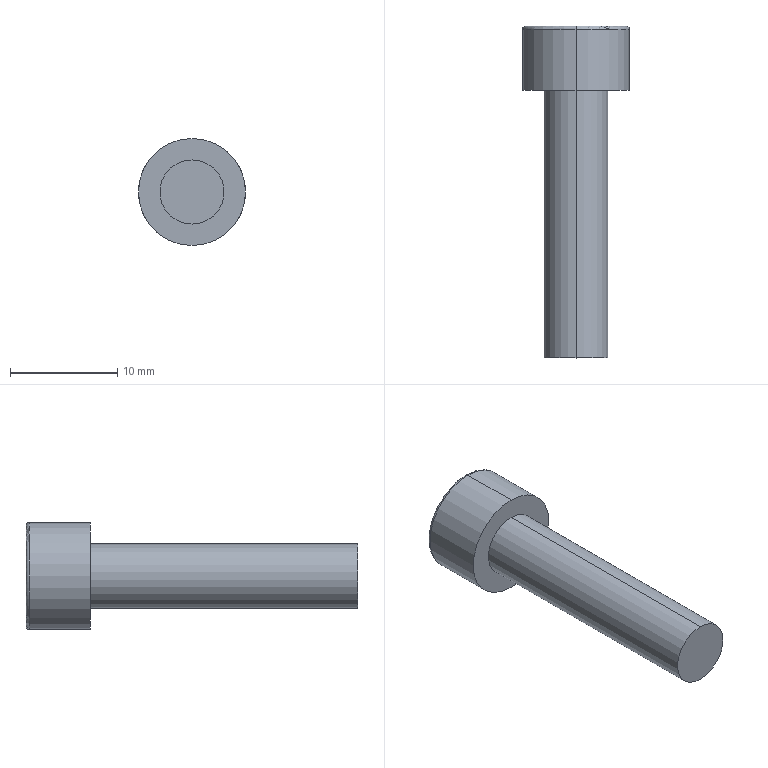Part | STEP file | M6 socket head cap screw simplified_M6x25 | 1 solid | 16 faces | box 10 x 31 x 10 mm | volume 1110 mm3 | plane 10 | cylinder 4 | torus 2 | commonest cylinder face diameters 6 x2 10 x2
STEP:
#1=CARTESIAN_POINT('',(0.,0.,0.));
#2=DIRECTION('',(0.,0.,1.));
#3=DIRECTION('',(1.,0.,0.));
#4=AXIS2_PLACEMENT_3D('',#1,#2,#3);
#5=CARTESIAN_POINT('',(0.,0.,4.7));
#6=VERTEX_POINT('',#5);
#7=CARTESIAN_POINT('',(0.,0.,-4.7));
#8=VERTEX_POINT('',#7);
#9=CARTESIAN_POINT('',(0.,0.,0.));
#10=DIRECTION('',(0.,1.,0.));
#11=DIRECTION('',(0.,0.,-1.));
#12=AXIS2_PLACEMENT_3D('',#9,#10,#11);
#13=CIRCLE('',#12,4.7);
#14=CARTESIAN_POINT('',(0.,-0.3,0.));
#15=DIRECTION('',(0.,-1.,0.));
#16=DIRECTION('',(0.,0.,-1.));
#17=AXIS2_PLACEMENT_3D('',#14,#15,#16);
#18=TOROIDAL_SURFACE('',#17,4.7,0.3);
#19=CARTESIAN_POINT('',(6.283,4.712));
#20=DIRECTION('',(-1.,0.));
#21=VECTOR('',#20,1.);
#22=LINE('',#19,#21);
#23=(GEOMETRIC_REPRESENTATION_CONTEXT(2)PARAMETRIC_REPRESENTATION_CONTEXT()REPRESENTATION_CONTEXT('',''));
#24=DEFINITIONAL_REPRESENTATION('',(#22),#23);
#25=PCURVE('',#18,#24);
#26=CARTESIAN_POINT('',(0.,0.,0.));
#27=DIRECTION('',(0.,-1.,0.));
#28=DIRECTION('',(0.,0.,-1.));
#29=AXIS2_PLACEMENT_3D('',#26,#27,#28);
#30=PLANE('',#29);
#31=CARTESIAN_POINT('',(4.7,0.));
#32=CARTESIAN_POINT('',(4.7,-8.141));
#33=CARTESIAN_POINT('',(-2.35,-4.07));
#34=CARTESIAN_POINT('',(-9.4,0.));
#35=CARTESIAN_POINT('',(-2.35,4.07));
#36=CARTESIAN_POINT('',(4.7,8.141));
#37=CARTESIAN_POINT('',(4.7,0.));
#38=(BOUNDED_CURVE()B_SPLINE_CURVE(2,(#31,#32,#33,#34,#35,#36,#37),.UNSPECIFIED.,.T.,.F.)B_SPLINE_CURVE_WITH_KNOTS((1,2,2,2,2,1),(-2.094,0.,2.094,4.189,6.283,8.378),.UNSPECIFIED.)CURVE()GEOMETRIC_REPRESENTATION_ITEM()RATIONAL_B_SPLINE_CURVE((1.,0.5,1.,0.5,1.,0.5,1.))REPRESENTATION_ITEM(''));
#39=(GEOMETRIC_REPRESENTATION_CONTEXT(2)PARAMETRIC_REPRESENTATION_CONTEXT()REPRESENTATION_CONTEXT('',''));
#40=DEFINITIONAL_REPRESENTATION('',(#38),#39);
#41=PCURVE('',#30,#40);
#42=SURFACE_CURVE('',#13,(#25,#41),.PCURVE_S1.);
#43=EDGE_CURVE('',#6,#8,#42,.T.);
#44=ORIENTED_EDGE('',*,*,#43,.F.);
#45=CARTESIAN_POINT('',(0.,-0.3,5.));
#46=VERTEX_POINT('',#45);
#47=CARTESIAN_POINT('',(0.,-0.3,4.7));
#48=DIRECTION('',(1.,0.,0.));
#49=DIRECTION('',(0.,0.,-1.));
#50=AXIS2_PLACEMENT_3D('',#47,#48,#49);
#51=CIRCLE('',#50,0.3);
#52=CARTESIAN_POINT('',(3.142,3.142));
#53=DIRECTION('',(0.,1.));
#54=VECTOR('',#53,1.);
#55=LINE('',#52,#54);
#56=(GEOMETRIC_REPRESENTATION_CONTEXT(2)PARAMETRIC_REPRESENTATION_CONTEXT()REPRESENTATION_CONTEXT('',''));
#57=DEFINITIONAL_REPRESENTATION('',(#55),#56);
#58=PCURVE('',#18,#57);
#59=CARTESIAN_POINT('',(0.,-0.3,0.));
#60=DIRECTION('',(0.,-1.,0.));
#61=DIRECTION('',(0.,0.,-1.));
#62=AXIS2_PLACEMENT_3D('',#59,#60,#61);
#63=TOROIDAL_SURFACE('',#62,4.7,0.3);
#64=CARTESIAN_POINT('',(3.142,3.142));
#65=DIRECTION('',(0.,1.));
#66=VECTOR('',#65,1.);
#67=LINE('',#64,#66);
#68=(GEOMETRIC_REPRESENTATION_CONTEXT(2)PARAMETRIC_REPRESENTATION_CONTEXT()REPRESENTATION_CONTEXT('',''));
#69=DEFINITIONAL_REPRESENTATION('',(#67),#68);
#70=PCURVE('',#63,#69);
#71=SURFACE_CURVE('',#51,(#58,#70),.PCURVE_S1.);
#72=EDGE_CURVE('',#6,#46,#71,.T.);
#73=ORIENTED_EDGE('',*,*,#72,.T.);
#74=CARTESIAN_POINT('',(0.,-0.3,-5.));
#75=VERTEX_POINT('',#74);
#76=CARTESIAN_POINT('',(0.,-0.3,0.));
#77=DIRECTION('',(0.,-1.,0.));
#78=DIRECTION('',(0.,0.,-1.));
#79=AXIS2_PLACEMENT_3D('',#76,#77,#78);
#80=CIRCLE('',#79,5.);
#81=CARTESIAN_POINT('',(0.,6.283));
#82=DIRECTION('',(1.,0.));
#83=VECTOR('',#82,1.);
#84=LINE('',#81,#83);
#85=(GEOMETRIC_REPRESENTATION_CONTEXT(2)PARAMETRIC_REPRESENTATION_CONTEXT()REPRESENTATION_CONTEXT('',''));
#86=DEFINITIONAL_REPRESENTATION('',(#84),#85);
#87=PCURVE('',#18,#86);
#88=CARTESIAN_POINT('',(0.,0.,0.));
#89=DIRECTION('',(0.,1.,0.));
#90=DIRECTION('',(0.,0.,1.));
#91=AXIS2_PLACEMENT_3D('',#88,#89,#90);
#92=CYLINDRICAL_SURFACE('',#91,5.);
#93=CARTESIAN_POINT('',(3.142,-0.3));
#94=DIRECTION('',(-1.,0.));
#95=VECTOR('',#94,1.);
#96=LINE('',#93,#95);
#97=(GEOMETRIC_REPRESENTATION_CONTEXT(2)PARAMETRIC_REPRESENTATION_CONTEXT()REPRESENTATION_CONTEXT('',''));
#98=DEFINITIONAL_REPRESENTATION('',(#96),#97);
#99=PCURVE('',#92,#98);
#100=SURFACE_CURVE('',#80,(#87,#99),.PCURVE_S1.);
#101=EDGE_CURVE('',#75,#46,#100,.T.);
#102=ORIENTED_EDGE('',*,*,#101,.F.);
#103=CARTESIAN_POINT('',(0.,-0.3,-4.7));
#104=DIRECTION('',(-1.,0.,0.));
#105=DIRECTION('',(0.,0.,1.));
#106=AXIS2_PLACEMENT_3D('',#103,#104,#105);
#107=CIRCLE('',#106,0.3);
#108=CARTESIAN_POINT('',(0.,3.142));
#109=DIRECTION('',(0.,1.));
#110=VECTOR('',#109,1.);
#111=LINE('',#108,#110);
#112=(GEOMETRIC_REPRESENTATION_CONTEXT(2)PARAMETRIC_REPRESENTATION_CONTEXT()REPRESENTATION_CONTEXT('',''));
#113=DEFINITIONAL_REPRESENTATION('',(#111),#112);
#114=PCURVE('',#18,#113);
#115=CARTESIAN_POINT('',(6.283,3.142));
#116=DIRECTION('',(0.,1.));
#117=VECTOR('',#116,1.);
#118=LINE('',#115,#117);
#119=(GEOMETRIC_REPRESENTATION_CONTEXT(2)PARAMETRIC_REPRESENTATION_CONTEXT()REPRESENTATION_CONTEXT('',''));
#120=DEFINITIONAL_REPRESENTATION('',(#118),#119);
#121=PCURVE('',#63,#120);
#122=SURFACE_CURVE('',#107,(#114,#121),.PCURVE_S1.);
#123=EDGE_CURVE('',#8,#75,#122,.T.);
#124=ORIENTED_EDGE('',*,*,#123,.F.);
#125=EDGE_LOOP('',(#44,#73,#102,#124));
#126=FACE_BOUND('',#125,.T.);
#127=ADVANCED_FACE('',(#126),#18,.T.);
#128=CARTESIAN_POINT('',(0.,-31.,3.));
#129=VERTEX_POINT('',#128);
#130=CARTESIAN_POINT('',(0.,-31.,-3.));
#131=VERTEX_POINT('',#130);
#132=CARTESIAN_POINT('',(0.,-31.,0.));
#133=DIRECTION('',(0.,1.,0.));
#134=DIRECTION('',(0.,0.,1.));
#135=AXIS2_PLACEMENT_3D('',#132,#133,#134);
#136=CIRCLE('',#135,3.);
#137=CARTESIAN_POINT('',(0.,0.,0.));
#138=DIRECTION('',(0.,1.,0.));
#139=DIRECTION('',(0.,0.,1.));
#140=AXIS2_PLACEMENT_3D('',#137,#138,#139);
#141=CYLINDRICAL_SURFACE('',#140,3.);
#142=CARTESIAN_POINT('',(0.,-31.));
#143=DIRECTION('',(1.,0.));
#144=VECTOR('',#143,1.);
#145=LINE('',#142,#144);
#146=(GEOMETRIC_REPRESENTATION_CONTEXT(2)PARAMETRIC_REPRESENTATION_CONTEXT()REPRESENTATION_CONTEXT('',''));
#147=DEFINITIONAL_REPRESENTATION('',(#145),#146);
#148=PCURVE('',#141,#147);
#149=CARTESIAN_POINT('',(3.,-31.,0.));
#150=DIRECTION('',(0.,1.,0.));
#151=DIRECTION('',(0.,0.,1.));
#152=AXIS2_PLACEMENT_3D('',#149,#150,#151);
#153=PLANE('',#152);
#154=CARTESIAN_POINT('',(0.,-3.));
#155=DIRECTION('',(1.,0.));
#156=AXIS2_PLACEMENT_2D('',#154,#155);
#157=CIRCLE('',#156,3.);
#158=(GEOMETRIC_REPRESENTATION_CONTEXT(2)PARAMETRIC_REPRESENTATION_CONTEXT()REPRESENTATION_CONTEXT('',''));
#159=DEFINITIONAL_REPRESENTATION('',(#157),#158);
#160=PCURVE('',#153,#159);
#161=SURFACE_CURVE('',#136,(#148,#160),.PCURVE_S1.);
#162=EDGE_CURVE('',#129,#131,#161,.T.);
#163=ORIENTED_EDGE('',*,*,#162,.T.);
#164=CARTESIAN_POINT('',(0.,-6.,-3.));
#165=VERTEX_POINT('',#164);
#166=CARTESIAN_POINT('',(0.,0.,-3.));
#167=DIRECTION('',(0.,1.,0.));
#168=VECTOR('',#167,1.);
#169=LINE('',#166,#168);
#170=CARTESIAN_POINT('',(3.142,0.));
#171=DIRECTION('',(0.,1.));
#172=VECTOR('',#171,1.);
#173=LINE('',#170,#172);
#174=(GEOMETRIC_REPRESENTATION_CONTEXT(2)PARAMETRIC_REPRESENTATION_CONTEXT()REPRESENTATION_CONTEXT('',''));
#175=DEFINITIONAL_REPRESENTATION('',(#173),#174);
#176=PCURVE('',#141,#175);
#177=CARTESIAN_POINT('',(0.,0.,0.));
#178=DIRECTION('',(0.,1.,0.));
#179=DIRECTION('',(0.,0.,1.));
#180=AXIS2_PLACEMENT_3D('',#177,#178,#179);
#181=CYLINDRICAL_SURFACE('',#180,3.);
#182=CARTESIAN_POINT('',(3.142,0.));
#183=DIRECTION('',(0.,1.));
#184=VECTOR('',#183,1.);
#185=LINE('',#182,#184);
#186=(GEOMETRIC_REPRESENTATION_CONTEXT(2)PARAMETRIC_REPRESENTATION_CONTEXT()REPRESENTATION_CONTEXT('',''));
#187=DEFINITIONAL_REPRESENTATION('',(#185),#186);
#188=PCURVE('',#181,#187);
#189=SURFACE_CURVE('',#169,(#176,#188),.PCURVE_S1.);
#190=EDGE_CURVE('',#131,#165,#189,.T.);
#191=ORIENTED_EDGE('',*,*,#190,.T.);
#192=CARTESIAN_POINT('',(0.,-6.,3.));
#193=VERTEX_POINT('',#192);
#194=CARTESIAN_POINT('',(0.,-6.,0.));
#195=DIRECTION('',(0.,1.,0.));
#196=DIRECTION('',(0.,0.,1.));
#197=AXIS2_PLACEMENT_3D('',#194,#195,#196);
#198=CIRCLE('',#197,3.);
#199=CARTESIAN_POINT('',(0.,-6.));
#200=DIRECTION('',(1.,0.));
#201=VECTOR('',#200,1.);
#202=LINE('',#199,#201);
#203=(GEOMETRIC_REPRESENTATION_CONTEXT(2)PARAMETRIC_REPRESENTATION_CONTEXT()REPRESENTATION_CONTEXT('',''));
#204=DEFINITIONAL_REPRESENTATION('',(#202),#203);
#205=PCURVE('',#141,#204);
#206=CARTESIAN_POINT('',(5.,-6.,0.));
#207=DIRECTION('',(0.,1.,0.));
#208=DIRECTION('',(0.,0.,1.));
#209=AXIS2_PLACEMENT_3D('',#206,#207,#208);
#210=PLANE('',#209);
#211=CARTESIAN_POINT('',(0.,-5.));
#212=DIRECTION('',(1.,0.));
#213=AXIS2_PLACEMENT_2D('',#211,#212);
#214=CIRCLE('',#213,3.);
#215=(GEOMETRIC_REPRESENTATION_CONTEXT(2)PARAMETRIC_REPRESENTATION_CONTEXT()REPRESENTATION_CONTEXT('',''));
#216=DEFINITIONAL_REPRESENTATION('',(#214),#215);
#217=PCURVE('',#210,#216);
#218=SURFACE_CURVE('',#198,(#205,#217),.PCURVE_S1.);
#219=EDGE_CURVE('',#193,#165,#218,.T.);
#220=ORIENTED_EDGE('',*,*,#219,.F.);
#221=CARTESIAN_POINT('',(0.,0.,3.));
#222=DIRECTION('',(0.,1.,0.));
#223=VECTOR('',#222,1.);
#224=LINE('',#221,#223);
#225=CARTESIAN_POINT('',(0.,0.));
#226=DIRECTION('',(0.,1.));
#227=VECTOR('',#226,1.);
#228=LINE('',#225,#227);
#229=(GEOMETRIC_REPRESENTATION_CONTEXT(2)PARAMETRIC_REPRESENTATION_CONTEXT()REPRESENTATION_CONTEXT('',''));
#230=DEFINITIONAL_REPRESENTATION('',(#228),#229);
#231=PCURVE('',#141,#230);
#232=CARTESIAN_POINT('',(6.283,0.));
#233=DIRECTION('',(0.,1.));
#234=VECTOR('',#233,1.);
#235=LINE('',#232,#234);
#236=(GEOMETRIC_REPRESENTATION_CONTEXT(2)PARAMETRIC_REPRESENTATION_CONTEXT()REPRESENTATION_CONTEXT('',''));
#237=DEFINITIONAL_REPRESENTATION('',(#235),#236);
#238=PCURVE('',#181,#237);
#239=SURFACE_CURVE('',#224,(#231,#238),.PCURVE_S1.);
#240=EDGE_CURVE('',#129,#193,#239,.T.);
#241=ORIENTED_EDGE('',*,*,#240,.F.);
#242=EDGE_LOOP('',(#163,#191,#220,#241));
#243=FACE_BOUND('',#242,.T.);
#244=ADVANCED_FACE('',(#243),#141,.T.);
#245=CARTESIAN_POINT('',(0.,-6.,5.));
#246=VERTEX_POINT('',#245);
#247=CARTESIAN_POINT('',(0.,-6.,-5.));
#248=VERTEX_POINT('',#247);
#249=CARTESIAN_POINT('',(0.,-6.,0.));
#250=DIRECTION('',(0.,1.,0.));
#251=DIRECTION('',(0.,0.,1.));
#252=AXIS2_PLACEMENT_3D('',#249,#250,#251);
#253=CIRCLE('',#252,5.);
#254=CARTESIAN_POINT('',(0.,-6.));
#255=DIRECTION('',(1.,0.));
#256=VECTOR('',#255,1.);
#257=LINE('',#254,#256);
#258=(GEOMETRIC_REPRESENTATION_CONTEXT(2)PARAMETRIC_REPRESENTATION_CONTEXT()REPRESENTATION_CONTEXT('',''));
#259=DEFINITIONAL_REPRESENTATION('',(#257),#258);
#260=PCURVE('',#92,#259);
#261=CARTESIAN_POINT('',(0.,-5.));
#262=DIRECTION('',(1.,0.));
#263=AXIS2_PLACEMENT_2D('',#261,#262);
#264=CIRCLE('',#263,5.);
#265=(GEOMETRIC_REPRESENTATION_CONTEXT(2)PARAMETRIC_REPRESENTATION_CONTEXT()REPRESENTATION_CONTEXT('',''));
#266=DEFINITIONAL_REPRESENTATION('',(#264),#265);
#267=PCURVE('',#210,#266);
#268=SURFACE_CURVE('',#253,(#260,#267),.PCURVE_S1.);
#269=EDGE_CURVE('',#246,#248,#268,.T.);
#270=ORIENTED_EDGE('',*,*,#269,.T.);
#271=CARTESIAN_POINT('',(0.,0.,-5.));
#272=DIRECTION('',(0.,1.,0.));
#273=VECTOR('',#272,1.);
#274=LINE('',#271,#273);
#275=CARTESIAN_POINT('',(3.142,0.));
#276=DIRECTION('',(0.,1.));
#277=VECTOR('',#276,1.);
#278=LINE('',#275,#277);
#279=(GEOMETRIC_REPRESENTATION_CONTEXT(2)PARAMETRIC_REPRESENTATION_CONTEXT()REPRESENTATION_CONTEXT('',''));
#280=DEFINITIONAL_REPRESENTATION('',(#278),#279);
#281=PCURVE('',#92,#280);
#282=CARTESIAN_POINT('',(0.,0.,0.));
#283=DIRECTION('',(0.,1.,0.));
#284=DIRECTION('',(0.,0.,1.));
#285=AXIS2_PLACEMENT_3D('',#282,#283,#284);
#286=CYLINDRICAL_SURFACE('',#285,5.);
#287=CARTESIAN_POINT('',(3.142,0.));
#288=DIRECTION('',(0.,1.));
#289=VECTOR('',#288,1.);
#290=LINE('',#287,#289);
#291=(GEOMETRIC_REPRESENTATION_CONTEXT(2)PARAMETRIC_REPRESENTATION_CONTEXT()REPRESENTATION_CONTEXT('',''));
#292=DEFINITIONAL_REPRESENTATION('',(#290),#291);
#293=PCURVE('',#286,#292);
#294=SURFACE_CURVE('',#274,(#281,#293),.PCURVE_S1.);
#295=EDGE_CURVE('',#248,#75,#294,.T.);
#296=ORIENTED_EDGE('',*,*,#295,.T.);
#297=ORIENTED_EDGE('',*,*,#101,.T.);
#298=CARTESIAN_POINT('',(0.,0.,5.));
#299=DIRECTION('',(0.,1.,0.));
#300=VECTOR('',#299,1.);
#301=LINE('',#298,#300);
#302=CARTESIAN_POINT('',(0.,0.));
#303=DIRECTION('',(0.,1.));
#304=VECTOR('',#303,1.);
#305=LINE('',#302,#304);
#306=(GEOMETRIC_REPRESENTATION_CONTEXT(2)PARAMETRIC_REPRESENTATION_CONTEXT()REPRESENTATION_CONTEXT('',''));
#307=DEFINITIONAL_REPRESENTATION('',(#305),#306);
#308=PCURVE('',#92,#307);
#309=CARTESIAN_POINT('',(6.283,0.));
#310=DIRECTION('',(0.,1.));
#311=VECTOR('',#310,1.);
#312=LINE('',#309,#311);
#313=(GEOMETRIC_REPRESENTATION_CONTEXT(2)PARAMETRIC_REPRESENTATION_CONTEXT()REPRESENTATION_CONTEXT('',''));
#314=DEFINITIONAL_REPRESENTATION('',(#312),#313);
#315=PCURVE('',#286,#314);
#316=SURFACE_CURVE('',#301,(#308,#315),.PCURVE_S1.);
#317=EDGE_CURVE('',#246,#46,#316,.T.);
#318=ORIENTED_EDGE('',*,*,#317,.F.);
#319=EDGE_LOOP('',(#270,#296,#297,#318));
#320=FACE_BOUND('',#319,.T.);
#321=ADVANCED_FACE('',(#320),#92,.T.);
#322=CARTESIAN_POINT('',(0.,0.,0.));
#323=DIRECTION('',(0.,1.,0.));
#324=DIRECTION('',(0.,0.,-1.));
#325=AXIS2_PLACEMENT_3D('',#322,#323,#324);
#326=CIRCLE('',#325,4.7);
#327=CARTESIAN_POINT('',(4.7,0.));
#328=CARTESIAN_POINT('',(4.7,-8.141));
#329=CARTESIAN_POINT('',(-2.35,-4.07));
#330=CARTESIAN_POINT('',(-9.4,0.));
#331=CARTESIAN_POINT('',(-2.35,4.07));
#332=CARTESIAN_POINT('',(4.7,8.141));
#333=CARTESIAN_POINT('',(4.7,0.));
#334=(BOUNDED_CURVE()B_SPLINE_CURVE(2,(#327,#328,#329,#330,#331,#332,#333),.UNSPECIFIED.,.T.,.F.)B_SPLINE_CURVE_WITH_KNOTS((1,2,2,2,2,1),(-2.094,0.,2.094,4.189,6.283,8.378),.UNSPECIFIED.)CURVE()GEOMETRIC_REPRESENTATION_ITEM()RATIONAL_B_SPLINE_CURVE((1.,0.5,1.,0.5,1.,0.5,1.))REPRESENTATION_ITEM(''));
#335=(GEOMETRIC_REPRESENTATION_CONTEXT(2)PARAMETRIC_REPRESENTATION_CONTEXT()REPRESENTATION_CONTEXT('',''));
#336=DEFINITIONAL_REPRESENTATION('',(#334),#335);
#337=PCURVE('',#30,#336);
#338=CARTESIAN_POINT('',(6.283,4.712));
#339=DIRECTION('',(-1.,0.));
#340=VECTOR('',#339,1.);
#341=LINE('',#338,#340);
#342=(GEOMETRIC_REPRESENTATION_CONTEXT(2)PARAMETRIC_REPRESENTATION_CONTEXT()REPRESENTATION_CONTEXT('',''));
#343=DEFINITIONAL_REPRESENTATION('',(#341),#342);
#344=PCURVE('',#63,#343);
#345=SURFACE_CURVE('',#326,(#337,#344),.PCURVE_S1.);
#346=EDGE_CURVE('',#8,#6,#345,.T.);
#347=ORIENTED_EDGE('',*,*,#346,.T.);
#348=ORIENTED_EDGE('',*,*,#43,.T.);
#349=EDGE_LOOP('',(#347,#348));
#350=FACE_BOUND('',#349,.T.);
#351=CARTESIAN_POINT('',(-2.944,0.,0.));
#352=VERTEX_POINT('',#351);
#353=CARTESIAN_POINT('',(-1.472,0.,2.55));
#354=VERTEX_POINT('',#353);
#355=CARTESIAN_POINT('',(-2.944,0.,0.));
#356=DIRECTION('',(0.5,0.,0.866));
#357=VECTOR('',#356,1.);
#358=LINE('',#355,#357);
#359=CARTESIAN_POINT('',(0.,-2.944));
#360=DIRECTION('',(-0.866,0.5));
#361=VECTOR('',#360,1.);
#362=LINE('',#359,#361);
#363=(GEOMETRIC_REPRESENTATION_CONTEXT(2)PARAMETRIC_REPRESENTATION_CONTEXT()REPRESENTATION_CONTEXT('',''));
#364=DEFINITIONAL_REPRESENTATION('',(#362),#363);
#365=PCURVE('',#30,#364);
#366=CARTESIAN_POINT('',(-2.944,-3.,0.));
#367=DIRECTION('',(-0.866,0.,0.5));
#368=DIRECTION('',(0.5,0.,0.866));
#369=AXIS2_PLACEMENT_3D('',#366,#367,#368);
#370=PLANE('',#369);
#371=CARTESIAN_POINT('',(0.,3.));
#372=DIRECTION('',(1.,0.));
#373=VECTOR('',#372,1.);
#374=LINE('',#371,#373);
#375=(GEOMETRIC_REPRESENTATION_CONTEXT(2)PARAMETRIC_REPRESENTATION_CONTEXT()REPRESENTATION_CONTEXT('',''));
#376=DEFINITIONAL_REPRESENTATION('',(#374),#375);
#377=PCURVE('',#370,#376);
#378=SURFACE_CURVE('',#358,(#365,#377),.PCURVE_S1.);
#379=EDGE_CURVE('',#352,#354,#378,.T.);
#380=ORIENTED_EDGE('',*,*,#379,.F.);
#381=CARTESIAN_POINT('',(-1.472,0.,-2.55));
#382=VERTEX_POINT('',#381);
#383=CARTESIAN_POINT('',(-1.472,0.,-2.55));
#384=DIRECTION('',(-0.5,0.,0.866));
#385=VECTOR('',#384,1.);
#386=LINE('',#383,#385);
#387=CARTESIAN_POINT('',(2.55,-1.472));
#388=DIRECTION('',(-0.866,-0.5));
#389=VECTOR('',#388,1.);
#390=LINE('',#387,#389);
#391=(GEOMETRIC_REPRESENTATION_CONTEXT(2)PARAMETRIC_REPRESENTATION_CONTEXT()REPRESENTATION_CONTEXT('',''));
#392=DEFINITIONAL_REPRESENTATION('',(#390),#391);
#393=PCURVE('',#30,#392);
#394=CARTESIAN_POINT('',(-1.472,-3.,-2.55));
#395=DIRECTION('',(-0.866,0.,-0.5));
#396=DIRECTION('',(-0.5,0.,0.866));
#397=AXIS2_PLACEMENT_3D('',#394,#395,#396);
#398=PLANE('',#397);
#399=CARTESIAN_POINT('',(0.,3.));
#400=DIRECTION('',(1.,0.));
#401=VECTOR('',#400,1.);
#402=LINE('',#399,#401);
#403=(GEOMETRIC_REPRESENTATION_CONTEXT(2)PARAMETRIC_REPRESENTATION_CONTEXT()REPRESENTATION_CONTEXT('',''));
#404=DEFINITIONAL_REPRESENTATION('',(#402),#403);
#405=PCURVE('',#398,#404);
#406=SURFACE_CURVE('',#386,(#393,#405),.PCURVE_S1.);
#407=EDGE_CURVE('',#382,#352,#406,.T.);
#408=ORIENTED_EDGE('',*,*,#407,.F.);
#409=CARTESIAN_POINT('',(1.472,0.,-2.55));
#410=VERTEX_POINT('',#409);
#411=CARTESIAN_POINT('',(1.472,0.,-2.55));
#412=DIRECTION('',(-1.,0.,0.));
#413=VECTOR('',#412,1.);
#414=LINE('',#411,#413);
#415=CARTESIAN_POINT('',(2.55,1.472));
#416=DIRECTION('',(0.,-1.));
#417=VECTOR('',#416,1.);
#418=LINE('',#415,#417);
#419=(GEOMETRIC_REPRESENTATION_CONTEXT(2)PARAMETRIC_REPRESENTATION_CONTEXT()REPRESENTATION_CONTEXT('',''));
#420=DEFINITIONAL_REPRESENTATION('',(#418),#419);
#421=PCURVE('',#30,#420);
#422=CARTESIAN_POINT('',(1.472,-3.,-2.55));
#423=DIRECTION('',(0.,0.,-1.));
#424=DIRECTION('',(-1.,0.,0.));
#425=AXIS2_PLACEMENT_3D('',#422,#423,#424);
#426=PLANE('',#425);
#427=CARTESIAN_POINT('',(0.,3.));
#428=DIRECTION('',(1.,0.));
#429=VECTOR('',#428,1.);
#430=LINE('',#427,#429);
#431=(GEOMETRIC_REPRESENTATION_CONTEXT(2)PARAMETRIC_REPRESENTATION_CONTEXT()REPRESENTATION_CONTEXT('',''));
#432=DEFINITIONAL_REPRESENTATION('',(#430),#431);
#433=PCURVE('',#426,#432);
#434=SURFACE_CURVE('',#414,(#421,#433),.PCURVE_S1.);
#435=EDGE_CURVE('',#410,#382,#434,.T.);
#436=ORIENTED_EDGE('',*,*,#435,.F.);
#437=CARTESIAN_POINT('',(2.944,0.,0.));
#438=VERTEX_POINT('',#437);
#439=CARTESIAN_POINT('',(2.944,0.,0.));
#440=DIRECTION('',(-0.5,0.,-0.866));
#441=VECTOR('',#440,1.);
#442=LINE('',#439,#441);
#443=CARTESIAN_POINT('',(0.,2.944));
#444=DIRECTION('',(0.866,-0.5));
#445=VECTOR('',#444,1.);
#446=LINE('',#443,#445);
#447=(GEOMETRIC_REPRESENTATION_CONTEXT(2)PARAMETRIC_REPRESENTATION_CONTEXT()REPRESENTATION_CONTEXT('',''));
#448=DEFINITIONAL_REPRESENTATION('',(#446),#447);
#449=PCURVE('',#30,#448);
#450=CARTESIAN_POINT('',(2.944,-3.,0.));
#451=DIRECTION('',(0.866,0.,-0.5));
#452=DIRECTION('',(-0.5,0.,-0.866));
#453=AXIS2_PLACEMENT_3D('',#450,#451,#452);
#454=PLANE('',#453);
#455=CARTESIAN_POINT('',(0.,3.));
#456=DIRECTION('',(1.,0.));
#457=VECTOR('',#456,1.);
#458=LINE('',#455,#457);
#459=(GEOMETRIC_REPRESENTATION_CONTEXT(2)PARAMETRIC_REPRESENTATION_CONTEXT()REPRESENTATION_CONTEXT('',''));
#460=DEFINITIONAL_REPRESENTATION('',(#458),#459);
#461=PCURVE('',#454,#460);
#462=SURFACE_CURVE('',#442,(#449,#461),.PCURVE_S1.);
#463=EDGE_CURVE('',#438,#410,#462,.T.);
#464=ORIENTED_EDGE('',*,*,#463,.F.);
#465=CARTESIAN_POINT('',(1.472,0.,2.55));
#466=VERTEX_POINT('',#465);
#467=CARTESIAN_POINT('',(1.472,0.,2.55));
#468=DIRECTION('',(0.5,0.,-0.866));
#469=VECTOR('',#468,1.);
#470=LINE('',#467,#469);
#471=CARTESIAN_POINT('',(-2.55,1.472));
#472=DIRECTION('',(0.866,0.5));
#473=VECTOR('',#472,1.);
#474=LINE('',#471,#473);
#475=(GEOMETRIC_REPRESENTATION_CONTEXT(2)PARAMETRIC_REPRESENTATION_CONTEXT()REPRESENTATION_CONTEXT('',''));
#476=DEFINITIONAL_REPRESENTATION('',(#474),#475);
#477=PCURVE('',#30,#476);
#478=CARTESIAN_POINT('',(1.472,-3.,2.55));
#479=DIRECTION('',(0.866,0.,0.5));
#480=DIRECTION('',(0.5,0.,-0.866));
#481=AXIS2_PLACEMENT_3D('',#478,#479,#480);
#482=PLANE('',#481);
#483=CARTESIAN_POINT('',(0.,3.));
#484=DIRECTION('',(1.,0.));
#485=VECTOR('',#484,1.);
#486=LINE('',#483,#485);
#487=(GEOMETRIC_REPRESENTATION_CONTEXT(2)PARAMETRIC_REPRESENTATION_CONTEXT()REPRESENTATION_CONTEXT('',''));
#488=DEFINITIONAL_REPRESENTATION('',(#486),#487);
#489=PCURVE('',#482,#488);
#490=SURFACE_CURVE('',#470,(#477,#489),.PCURVE_S1.);
#491=EDGE_CURVE('',#466,#438,#490,.T.);
#492=ORIENTED_EDGE('',*,*,#491,.F.);
#493=CARTESIAN_POINT('',(-1.472,0.,2.55));
#494=DIRECTION('',(1.,0.,0.));
#495=VECTOR('',#494,1.);
#496=LINE('',#493,#495);
#497=CARTESIAN_POINT('',(-2.55,-1.472));
#498=DIRECTION('',(0.,1.));
#499=VECTOR('',#498,1.);
#500=LINE('',#497,#499);
#501=(GEOMETRIC_REPRESENTATION_CONTEXT(2)PARAMETRIC_REPRESENTATION_CONTEXT()REPRESENTATION_CONTEXT('',''));
#502=DEFINITIONAL_REPRESENTATION('',(#500),#501);
#503=PCURVE('',#30,#502);
#504=CARTESIAN_POINT('',(-1.472,-3.,2.55));
#505=DIRECTION('',(0.,0.,1.));
#506=DIRECTION('',(1.,0.,0.));
#507=AXIS2_PLACEMENT_3D('',#504,#505,#506);
#508=PLANE('',#507);
#509=CARTESIAN_POINT('',(0.,3.));
#510=DIRECTION('',(1.,0.));
#511=VECTOR('',#510,1.);
#512=LINE('',#509,#511);
#513=(GEOMETRIC_REPRESENTATION_CONTEXT(2)PARAMETRIC_REPRESENTATION_CONTEXT()REPRESENTATION_CONTEXT('',''));
#514=DEFINITIONAL_REPRESENTATION('',(#512),#513);
#515=PCURVE('',#508,#514);
#516=SURFACE_CURVE('',#496,(#503,#515),.PCURVE_S1.);
#517=EDGE_CURVE('',#354,#466,#516,.T.);
#518=ORIENTED_EDGE('',*,*,#517,.F.);
#519=EDGE_LOOP('',(#380,#408,#436,#464,#492,#518));
#520=FACE_BOUND('',#519,.T.);
#521=ADVANCED_FACE('',(#350,#520),#30,.F.);
#522=ORIENTED_EDGE('',*,*,#295,.F.);
#523=CARTESIAN_POINT('',(0.,-6.,0.));
#524=DIRECTION('',(0.,1.,0.));
#525=DIRECTION('',(0.,0.,1.));
#526=AXIS2_PLACEMENT_3D('',#523,#524,#525);
#527=CIRCLE('',#526,5.);
#528=CARTESIAN_POINT('',(0.,-6.));
#529=DIRECTION('',(1.,0.));
#530=VECTOR('',#529,1.);
#531=LINE('',#528,#530);
#532=(GEOMETRIC_REPRESENTATION_CONTEXT(2)PARAMETRIC_REPRESENTATION_CONTEXT()REPRESENTATION_CONTEXT('',''));
#533=DEFINITIONAL_REPRESENTATION('',(#531),#532);
#534=PCURVE('',#286,#533);
#535=CARTESIAN_POINT('',(0.,-5.));
#536=DIRECTION('',(1.,0.));
#537=AXIS2_PLACEMENT_2D('',#535,#536);
#538=CIRCLE('',#537,5.);
#539=(GEOMETRIC_REPRESENTATION_CONTEXT(2)PARAMETRIC_REPRESENTATION_CONTEXT()REPRESENTATION_CONTEXT('',''));
#540=DEFINITIONAL_REPRESENTATION('',(#538),#539);
#541=PCURVE('',#210,#540);
#542=SURFACE_CURVE('',#527,(#534,#541),.PCURVE_S1.);
#543=EDGE_CURVE('',#248,#246,#542,.T.);
#544=ORIENTED_EDGE('',*,*,#543,.T.);
#545=ORIENTED_EDGE('',*,*,#317,.T.);
#546=CARTESIAN_POINT('',(0.,-0.3,0.));
#547=DIRECTION('',(0.,-1.,0.));
#548=DIRECTION('',(0.,0.,-1.));
#549=AXIS2_PLACEMENT_3D('',#546,#547,#548);
#550=CIRCLE('',#549,5.);
#551=CARTESIAN_POINT('',(9.425,-0.3));
#552=DIRECTION('',(-1.,0.));
#553=VECTOR('',#552,1.);
#554=LINE('',#551,#553);
#555=(GEOMETRIC_REPRESENTATION_CONTEXT(2)PARAMETRIC_REPRESENTATION_CONTEXT()REPRESENTATION_CONTEXT('',''));
#556=DEFINITIONAL_REPRESENTATION('',(#554),#555);
#557=PCURVE('',#286,#556);
#558=CARTESIAN_POINT('',(0.,6.283));
#559=DIRECTION('',(1.,0.));
#560=VECTOR('',#559,1.);
#561=LINE('',#558,#560);
#562=(GEOMETRIC_REPRESENTATION_CONTEXT(2)PARAMETRIC_REPRESENTATION_CONTEXT()REPRESENTATION_CONTEXT('',''));
#563=DEFINITIONAL_REPRESENTATION('',(#561),#562);
#564=PCURVE('',#63,#563);
#565=SURFACE_CURVE('',#550,(#557,#564),.PCURVE_S1.);
#566=EDGE_CURVE('',#46,#75,#565,.T.);
#567=ORIENTED_EDGE('',*,*,#566,.T.);
#568=EDGE_LOOP('',(#522,#544,#545,#567));
#569=FACE_BOUND('',#568,.T.);
#570=ADVANCED_FACE('',(#569),#286,.T.);
#571=ORIENTED_EDGE('',*,*,#269,.F.);
#572=ORIENTED_EDGE('',*,*,#543,.F.);
#573=EDGE_LOOP('',(#571,#572));
#574=FACE_BOUND('',#573,.T.);
#575=ORIENTED_EDGE('',*,*,#219,.T.);
#576=CARTESIAN_POINT('',(0.,-6.,0.));
#577=DIRECTION('',(0.,1.,0.));
#578=DIRECTION('',(0.,0.,1.));
#579=AXIS2_PLACEMENT_3D('',#576,#577,#578);
#580=CIRCLE('',#579,3.);
#581=CARTESIAN_POINT('',(0.,-5.));
#582=DIRECTION('',(1.,0.));
#583=AXIS2_PLACEMENT_2D('',#581,#582);
#584=CIRCLE('',#583,3.);
#585=(GEOMETRIC_REPRESENTATION_CONTEXT(2)PARAMETRIC_REPRESENTATION_CONTEXT()REPRESENTATION_CONTEXT('',''));
#586=DEFINITIONAL_REPRESENTATION('',(#584),#585);
#587=PCURVE('',#210,#586);
#588=CARTESIAN_POINT('',(0.,-6.));
#589=DIRECTION('',(1.,0.));
#590=VECTOR('',#589,1.);
#591=LINE('',#588,#590);
#592=(GEOMETRIC_REPRESENTATION_CONTEXT(2)PARAMETRIC_REPRESENTATION_CONTEXT()REPRESENTATION_CONTEXT('',''));
#593=DEFINITIONAL_REPRESENTATION('',(#591),#592);
#594=PCURVE('',#181,#593);
#595=SURFACE_CURVE('',#580,(#587,#594),.PCURVE_S1.);
#596=EDGE_CURVE('',#165,#193,#595,.T.);
#597=ORIENTED_EDGE('',*,*,#596,.T.);
#598=EDGE_LOOP('',(#575,#597));
#599=FACE_BOUND('',#598,.T.);
#600=ADVANCED_FACE('',(#574,#599),#210,.F.);
#601=ORIENTED_EDGE('',*,*,#190,.F.);
#602=CARTESIAN_POINT('',(0.,-31.,0.));
#603=DIRECTION('',(0.,1.,0.));
#604=DIRECTION('',(0.,0.,1.));
#605=AXIS2_PLACEMENT_3D('',#602,#603,#604);
#606=CIRCLE('',#605,3.);
#607=CARTESIAN_POINT('',(0.,-31.));
#608=DIRECTION('',(1.,0.));
#609=VECTOR('',#608,1.);
#610=LINE('',#607,#609);
#611=(GEOMETRIC_REPRESENTATION_CONTEXT(2)PARAMETRIC_REPRESENTATION_CONTEXT()REPRESENTATION_CONTEXT('',''));
#612=DEFINITIONAL_REPRESENTATION('',(#610),#611);
#613=PCURVE('',#181,#612);
#614=CARTESIAN_POINT('',(0.,-3.));
#615=DIRECTION('',(1.,0.));
#616=AXIS2_PLACEMENT_2D('',#614,#615);
#617=CIRCLE('',#616,3.);
#618=(GEOMETRIC_REPRESENTATION_CONTEXT(2)PARAMETRIC_REPRESENTATION_CONTEXT()REPRESENTATION_CONTEXT('',''));
#619=DEFINITIONAL_REPRESENTATION('',(#617),#618);
#620=PCURVE('',#153,#619);
#621=SURFACE_CURVE('',#606,(#613,#620),.PCURVE_S1.);
#622=EDGE_CURVE('',#131,#129,#621,.T.);
#623=ORIENTED_EDGE('',*,*,#622,.T.);
#624=ORIENTED_EDGE('',*,*,#240,.T.);
#625=ORIENTED_EDGE('',*,*,#596,.F.);
#626=EDGE_LOOP('',(#601,#623,#624,#625));
#627=FACE_BOUND('',#626,.T.);
#628=ADVANCED_FACE('',(#627),#181,.T.);
#629=ORIENTED_EDGE('',*,*,#162,.F.);
#630=ORIENTED_EDGE('',*,*,#622,.F.);
#631=EDGE_LOOP('',(#629,#630));
#632=FACE_BOUND('',#631,.T.);
#633=ADVANCED_FACE('',(#632),#153,.F.);
#634=ORIENTED_EDGE('',*,*,#407,.T.);
#635=CARTESIAN_POINT('',(-2.944,-3.,0.));
#636=VERTEX_POINT('',#635);
#637=CARTESIAN_POINT('',(-2.944,-3.,0.));
#638=DIRECTION('',(0.,1.,0.));
#639=VECTOR('',#638,1.);
#640=LINE('',#637,#639);
#641=CARTESIAN_POINT('',(2.944,0.));
#642=DIRECTION('',(0.,1.));
#643=VECTOR('',#642,1.);
#644=LINE('',#641,#643);
#645=(GEOMETRIC_REPRESENTATION_CONTEXT(2)PARAMETRIC_REPRESENTATION_CONTEXT()REPRESENTATION_CONTEXT('',''));
#646=DEFINITIONAL_REPRESENTATION('',(#644),#645);
#647=PCURVE('',#398,#646);
#648=CARTESIAN_POINT('',(0.,0.));
#649=DIRECTION('',(0.,1.));
#650=VECTOR('',#649,1.);
#651=LINE('',#648,#650);
#652=(GEOMETRIC_REPRESENTATION_CONTEXT(2)PARAMETRIC_REPRESENTATION_CONTEXT()REPRESENTATION_CONTEXT('',''));
#653=DEFINITIONAL_REPRESENTATION('',(#651),#652);
#654=PCURVE('',#370,#653);
#655=SURFACE_CURVE('',#640,(#647,#654),.PCURVE_S1.);
#656=EDGE_CURVE('',#636,#352,#655,.T.);
#657=ORIENTED_EDGE('',*,*,#656,.F.);
#658=CARTESIAN_POINT('',(-1.472,-3.,-2.55));
#659=VERTEX_POINT('',#658);
#660=CARTESIAN_POINT('',(-1.472,-3.,-2.55));
#661=DIRECTION('',(-0.5,0.,0.866));
#662=VECTOR('',#661,1.);
#663=LINE('',#660,#662);
#664=CARTESIAN_POINT('',(0.,0.));
#665=DIRECTION('',(1.,0.));
#666=VECTOR('',#665,1.);
#667=LINE('',#664,#666);
#668=(GEOMETRIC_REPRESENTATION_CONTEXT(2)PARAMETRIC_REPRESENTATION_CONTEXT()REPRESENTATION_CONTEXT('',''));
#669=DEFINITIONAL_REPRESENTATION('',(#667),#668);
#670=PCURVE('',#398,#669);
#671=CARTESIAN_POINT('',(-2.944,-3.,0.));
#672=DIRECTION('',(0.,1.,0.));
#673=DIRECTION('',(0.,0.,1.));
#674=AXIS2_PLACEMENT_3D('',#671,#672,#673);
#675=PLANE('',#674);
#676=CARTESIAN_POINT('',(-2.55,1.472));
#677=DIRECTION('',(0.866,-0.5));
#678=VECTOR('',#677,1.);
#679=LINE('',#676,#678);
#680=(GEOMETRIC_REPRESENTATION_CONTEXT(2)PARAMETRIC_REPRESENTATION_CONTEXT()REPRESENTATION_CONTEXT('',''));
#681=DEFINITIONAL_REPRESENTATION('',(#679),#680);
#682=PCURVE('',#675,#681);
#683=SURFACE_CURVE('',#663,(#670,#682),.PCURVE_S1.);
#684=EDGE_CURVE('',#659,#636,#683,.T.);
#685=ORIENTED_EDGE('',*,*,#684,.F.);
#686=CARTESIAN_POINT('',(-1.472,-3.,-2.55));
#687=DIRECTION('',(0.,1.,0.));
#688=VECTOR('',#687,1.);
#689=LINE('',#686,#688);
#690=CARTESIAN_POINT('',(0.,0.));
#691=DIRECTION('',(0.,1.));
#692=VECTOR('',#691,1.);
#693=LINE('',#690,#692);
#694=(GEOMETRIC_REPRESENTATION_CONTEXT(2)PARAMETRIC_REPRESENTATION_CONTEXT()REPRESENTATION_CONTEXT('',''));
#695=DEFINITIONAL_REPRESENTATION('',(#693),#694);
#696=PCURVE('',#398,#695);
#697=CARTESIAN_POINT('',(2.944,0.));
#698=DIRECTION('',(0.,1.));
#699=VECTOR('',#698,1.);
#700=LINE('',#697,#699);
#701=(GEOMETRIC_REPRESENTATION_CONTEXT(2)PARAMETRIC_REPRESENTATION_CONTEXT()REPRESENTATION_CONTEXT('',''));
#702=DEFINITIONAL_REPRESENTATION('',(#700),#701);
#703=PCURVE('',#426,#702);
#704=SURFACE_CURVE('',#689,(#696,#703),.PCURVE_S1.);
#705=EDGE_CURVE('',#659,#382,#704,.T.);
#706=ORIENTED_EDGE('',*,*,#705,.T.);
#707=EDGE_LOOP('',(#634,#657,#685,#706));
#708=FACE_BOUND('',#707,.T.);
#709=ADVANCED_FACE('',(#708),#398,.F.);
#710=ORIENTED_EDGE('',*,*,#435,.T.);
#711=ORIENTED_EDGE('',*,*,#705,.F.);
#712=CARTESIAN_POINT('',(1.472,-3.,-2.55));
#713=VERTEX_POINT('',#712);
#714=CARTESIAN_POINT('',(1.472,-3.,-2.55));
#715=DIRECTION('',(-1.,0.,0.));
#716=VECTOR('',#715,1.);
#717=LINE('',#714,#716);
#718=CARTESIAN_POINT('',(0.,0.));
#719=DIRECTION('',(1.,0.));
#720=VECTOR('',#719,1.);
#721=LINE('',#718,#720);
#722=(GEOMETRIC_REPRESENTATION_CONTEXT(2)PARAMETRIC_REPRESENTATION_CONTEXT()REPRESENTATION_CONTEXT('',''));
#723=DEFINITIONAL_REPRESENTATION('',(#721),#722);
#724=PCURVE('',#426,#723);
#725=CARTESIAN_POINT('',(-2.55,4.417));
#726=DIRECTION('',(0.,-1.));
#727=VECTOR('',#726,1.);
#728=LINE('',#725,#727);
#729=(GEOMETRIC_REPRESENTATION_CONTEXT(2)PARAMETRIC_REPRESENTATION_CONTEXT()REPRESENTATION_CONTEXT('',''));
#730=DEFINITIONAL_REPRESENTATION('',(#728),#729);
#731=PCURVE('',#675,#730);
#732=SURFACE_CURVE('',#717,(#724,#731),.PCURVE_S1.);
#733=EDGE_CURVE('',#713,#659,#732,.T.);
#734=ORIENTED_EDGE('',*,*,#733,.F.);
#735=CARTESIAN_POINT('',(1.472,-3.,-2.55));
#736=DIRECTION('',(0.,1.,0.));
#737=VECTOR('',#736,1.);
#738=LINE('',#735,#737);
#739=CARTESIAN_POINT('',(0.,0.));
#740=DIRECTION('',(0.,1.));
#741=VECTOR('',#740,1.);
#742=LINE('',#739,#741);
#743=(GEOMETRIC_REPRESENTATION_CONTEXT(2)PARAMETRIC_REPRESENTATION_CONTEXT()REPRESENTATION_CONTEXT('',''));
#744=DEFINITIONAL_REPRESENTATION('',(#742),#743);
#745=PCURVE('',#426,#744);
#746=CARTESIAN_POINT('',(2.944,0.));
#747=DIRECTION('',(0.,1.));
#748=VECTOR('',#747,1.);
#749=LINE('',#746,#748);
#750=(GEOMETRIC_REPRESENTATION_CONTEXT(2)PARAMETRIC_REPRESENTATION_CONTEXT()REPRESENTATION_CONTEXT('',''));
#751=DEFINITIONAL_REPRESENTATION('',(#749),#750);
#752=PCURVE('',#454,#751);
#753=SURFACE_CURVE('',#738,(#745,#752),.PCURVE_S1.);
#754=EDGE_CURVE('',#713,#410,#753,.T.);
#755=ORIENTED_EDGE('',*,*,#754,.T.);
#756=EDGE_LOOP('',(#710,#711,#734,#755));
#757=FACE_BOUND('',#756,.T.);
#758=ADVANCED_FACE('',(#757),#426,.F.);
#759=ORIENTED_EDGE('',*,*,#463,.T.);
#760=ORIENTED_EDGE('',*,*,#754,.F.);
#761=CARTESIAN_POINT('',(2.944,-3.,0.));
#762=VERTEX_POINT('',#761);
#763=CARTESIAN_POINT('',(2.944,-3.,0.));
#764=DIRECTION('',(-0.5,0.,-0.866));
#765=VECTOR('',#764,1.);
#766=LINE('',#763,#765);
#767=CARTESIAN_POINT('',(0.,0.));
#768=DIRECTION('',(1.,0.));
#769=VECTOR('',#768,1.);
#770=LINE('',#767,#769);
#771=(GEOMETRIC_REPRESENTATION_CONTEXT(2)PARAMETRIC_REPRESENTATION_CONTEXT()REPRESENTATION_CONTEXT('',''));
#772=DEFINITIONAL_REPRESENTATION('',(#770),#771);
#773=PCURVE('',#454,#772);
#774=CARTESIAN_POINT('',(0.,5.889));
#775=DIRECTION('',(-0.866,-0.5));
#776=VECTOR('',#775,1.);
#777=LINE('',#774,#776);
#778=(GEOMETRIC_REPRESENTATION_CONTEXT(2)PARAMETRIC_REPRESENTATION_CONTEXT()REPRESENTATION_CONTEXT('',''));
#779=DEFINITIONAL_REPRESENTATION('',(#777),#778);
#780=PCURVE('',#675,#779);
#781=SURFACE_CURVE('',#766,(#773,#780),.PCURVE_S1.);
#782=EDGE_CURVE('',#762,#713,#781,.T.);
#783=ORIENTED_EDGE('',*,*,#782,.F.);
#784=CARTESIAN_POINT('',(2.944,-3.,0.));
#785=DIRECTION('',(0.,1.,0.));
#786=VECTOR('',#785,1.);
#787=LINE('',#784,#786);
#788=CARTESIAN_POINT('',(0.,0.));
#789=DIRECTION('',(0.,1.));
#790=VECTOR('',#789,1.);
#791=LINE('',#788,#790);
#792=(GEOMETRIC_REPRESENTATION_CONTEXT(2)PARAMETRIC_REPRESENTATION_CONTEXT()REPRESENTATION_CONTEXT('',''));
#793=DEFINITIONAL_REPRESENTATION('',(#791),#792);
#794=PCURVE('',#454,#793);
#795=CARTESIAN_POINT('',(2.944,0.));
#796=DIRECTION('',(0.,1.));
#797=VECTOR('',#796,1.);
#798=LINE('',#795,#797);
#799=(GEOMETRIC_REPRESENTATION_CONTEXT(2)PARAMETRIC_REPRESENTATION_CONTEXT()REPRESENTATION_CONTEXT('',''));
#800=DEFINITIONAL_REPRESENTATION('',(#798),#799);
#801=PCURVE('',#482,#800);
#802=SURFACE_CURVE('',#787,(#794,#801),.PCURVE_S1.);
#803=EDGE_CURVE('',#762,#438,#802,.T.);
#804=ORIENTED_EDGE('',*,*,#803,.T.);
#805=EDGE_LOOP('',(#759,#760,#783,#804));
#806=FACE_BOUND('',#805,.T.);
#807=ADVANCED_FACE('',(#806),#454,.F.);
#808=ORIENTED_EDGE('',*,*,#491,.T.);
#809=ORIENTED_EDGE('',*,*,#803,.F.);
#810=CARTESIAN_POINT('',(1.472,-3.,2.55));
#811=VERTEX_POINT('',#810);
#812=CARTESIAN_POINT('',(1.472,-3.,2.55));
#813=DIRECTION('',(0.5,0.,-0.866));
#814=VECTOR('',#813,1.);
#815=LINE('',#812,#814);
#816=CARTESIAN_POINT('',(0.,0.));
#817=DIRECTION('',(1.,0.));
#818=VECTOR('',#817,1.);
#819=LINE('',#816,#818);
#820=(GEOMETRIC_REPRESENTATION_CONTEXT(2)PARAMETRIC_REPRESENTATION_CONTEXT()REPRESENTATION_CONTEXT('',''));
#821=DEFINITIONAL_REPRESENTATION('',(#819),#820);
#822=PCURVE('',#482,#821);
#823=CARTESIAN_POINT('',(2.55,4.417));
#824=DIRECTION('',(-0.866,0.5));
#825=VECTOR('',#824,1.);
#826=LINE('',#823,#825);
#827=(GEOMETRIC_REPRESENTATION_CONTEXT(2)PARAMETRIC_REPRESENTATION_CONTEXT()REPRESENTATION_CONTEXT('',''));
#828=DEFINITIONAL_REPRESENTATION('',(#826),#827);
#829=PCURVE('',#675,#828);
#830=SURFACE_CURVE('',#815,(#822,#829),.PCURVE_S1.);
#831=EDGE_CURVE('',#811,#762,#830,.T.);
#832=ORIENTED_EDGE('',*,*,#831,.F.);
#833=CARTESIAN_POINT('',(1.472,-3.,2.55));
#834=DIRECTION('',(0.,1.,0.));
#835=VECTOR('',#834,1.);
#836=LINE('',#833,#835);
#837=CARTESIAN_POINT('',(0.,0.));
#838=DIRECTION('',(0.,1.));
#839=VECTOR('',#838,1.);
#840=LINE('',#837,#839);
#841=(GEOMETRIC_REPRESENTATION_CONTEXT(2)PARAMETRIC_REPRESENTATION_CONTEXT()REPRESENTATION_CONTEXT('',''));
#842=DEFINITIONAL_REPRESENTATION('',(#840),#841);
#843=PCURVE('',#482,#842);
#844=CARTESIAN_POINT('',(2.944,0.));
#845=DIRECTION('',(0.,1.));
#846=VECTOR('',#845,1.);
#847=LINE('',#844,#846);
#848=(GEOMETRIC_REPRESENTATION_CONTEXT(2)PARAMETRIC_REPRESENTATION_CONTEXT()REPRESENTATION_CONTEXT('',''));
#849=DEFINITIONAL_REPRESENTATION('',(#847),#848);
#850=PCURVE('',#508,#849);
#851=SURFACE_CURVE('',#836,(#843,#850),.PCURVE_S1.);
#852=EDGE_CURVE('',#811,#466,#851,.T.);
#853=ORIENTED_EDGE('',*,*,#852,.T.);
#854=EDGE_LOOP('',(#808,#809,#832,#853));
#855=FACE_BOUND('',#854,.T.);
#856=ADVANCED_FACE('',(#855),#482,.F.);
#857=ORIENTED_EDGE('',*,*,#517,.T.);
#858=ORIENTED_EDGE('',*,*,#852,.F.);
#859=CARTESIAN_POINT('',(-1.472,-3.,2.55));
#860=VERTEX_POINT('',#859);
#861=CARTESIAN_POINT('',(-1.472,-3.,2.55));
#862=DIRECTION('',(1.,0.,0.));
#863=VECTOR('',#862,1.);
#864=LINE('',#861,#863);
#865=CARTESIAN_POINT('',(0.,0.));
#866=DIRECTION('',(1.,0.));
#867=VECTOR('',#866,1.);
#868=LINE('',#865,#867);
#869=(GEOMETRIC_REPRESENTATION_CONTEXT(2)PARAMETRIC_REPRESENTATION_CONTEXT()REPRESENTATION_CONTEXT('',''));
#870=DEFINITIONAL_REPRESENTATION('',(#868),#869);
#871=PCURVE('',#508,#870);
#872=CARTESIAN_POINT('',(2.55,1.472));
#873=DIRECTION('',(0.,1.));
#874=VECTOR('',#873,1.);
#875=LINE('',#872,#874);
#876=(GEOMETRIC_REPRESENTATION_CONTEXT(2)PARAMETRIC_REPRESENTATION_CONTEXT()REPRESENTATION_CONTEXT('',''));
#877=DEFINITIONAL_REPRESENTATION('',(#875),#876);
#878=PCURVE('',#675,#877);
#879=SURFACE_CURVE('',#864,(#871,#878),.PCURVE_S1.);
#880=EDGE_CURVE('',#860,#811,#879,.T.);
#881=ORIENTED_EDGE('',*,*,#880,.F.);
#882=CARTESIAN_POINT('',(-1.472,-3.,2.55));
#883=DIRECTION('',(0.,1.,0.));
#884=VECTOR('',#883,1.);
#885=LINE('',#882,#884);
#886=CARTESIAN_POINT('',(0.,0.));
#887=DIRECTION('',(0.,1.));
#888=VECTOR('',#887,1.);
#889=LINE('',#886,#888);
#890=(GEOMETRIC_REPRESENTATION_CONTEXT(2)PARAMETRIC_REPRESENTATION_CONTEXT()REPRESENTATION_CONTEXT('',''));
#891=DEFINITIONAL_REPRESENTATION('',(#889),#890);
#892=PCURVE('',#508,#891);
#893=CARTESIAN_POINT('',(2.944,0.));
#894=DIRECTION('',(0.,1.));
#895=VECTOR('',#894,1.);
#896=LINE('',#893,#895);
#897=(GEOMETRIC_REPRESENTATION_CONTEXT(2)PARAMETRIC_REPRESENTATION_CONTEXT()REPRESENTATION_CONTEXT('',''));
#898=DEFINITIONAL_REPRESENTATION('',(#896),#897);
#899=PCURVE('',#370,#898);
#900=SURFACE_CURVE('',#885,(#892,#899),.PCURVE_S1.);
#901=EDGE_CURVE('',#860,#354,#900,.T.);
#902=ORIENTED_EDGE('',*,*,#901,.T.);
#903=EDGE_LOOP('',(#857,#858,#881,#902));
#904=FACE_BOUND('',#903,.T.);
#905=ADVANCED_FACE('',(#904),#508,.F.);
#906=ORIENTED_EDGE('',*,*,#379,.T.);
#907=ORIENTED_EDGE('',*,*,#901,.F.);
#908=CARTESIAN_POINT('',(-2.944,-3.,0.));
#909=DIRECTION('',(0.5,0.,0.866));
#910=VECTOR('',#909,1.);
#911=LINE('',#908,#910);
#912=CARTESIAN_POINT('',(0.,0.));
#913=DIRECTION('',(1.,0.));
#914=VECTOR('',#913,1.);
#915=LINE('',#912,#914);
#916=(GEOMETRIC_REPRESENTATION_CONTEXT(2)PARAMETRIC_REPRESENTATION_CONTEXT()REPRESENTATION_CONTEXT('',''));
#917=DEFINITIONAL_REPRESENTATION('',(#915),#916);
#918=PCURVE('',#370,#917);
#919=CARTESIAN_POINT('',(0.,0.));
#920=DIRECTION('',(0.866,0.5));
#921=VECTOR('',#920,1.);
#922=LINE('',#919,#921);
#923=(GEOMETRIC_REPRESENTATION_CONTEXT(2)PARAMETRIC_REPRESENTATION_CONTEXT()REPRESENTATION_CONTEXT('',''));
#924=DEFINITIONAL_REPRESENTATION('',(#922),#923);
#925=PCURVE('',#675,#924);
#926=SURFACE_CURVE('',#911,(#918,#925),.PCURVE_S1.);
#927=EDGE_CURVE('',#636,#860,#926,.T.);
#928=ORIENTED_EDGE('',*,*,#927,.F.);
#929=ORIENTED_EDGE('',*,*,#656,.T.);
#930=EDGE_LOOP('',(#906,#907,#928,#929));
#931=FACE_BOUND('',#930,.T.);
#932=ADVANCED_FACE('',(#931),#370,.F.);
#933=ORIENTED_EDGE('',*,*,#684,.T.);
#934=ORIENTED_EDGE('',*,*,#927,.T.);
#935=ORIENTED_EDGE('',*,*,#880,.T.);
#936=ORIENTED_EDGE('',*,*,#831,.T.);
#937=ORIENTED_EDGE('',*,*,#782,.T.);
#938=ORIENTED_EDGE('',*,*,#733,.T.);
#939=EDGE_LOOP('',(#933,#934,#935,#936,#937,#938));
#940=FACE_BOUND('',#939,.T.);
#941=ADVANCED_FACE('',(#940),#675,.T.);
#942=ORIENTED_EDGE('',*,*,#72,.F.);
#943=ORIENTED_EDGE('',*,*,#346,.F.);
#944=ORIENTED_EDGE('',*,*,#123,.T.);
#945=ORIENTED_EDGE('',*,*,#566,.F.);
#946=EDGE_LOOP('',(#942,#943,#944,#945));
#947=FACE_BOUND('',#946,.T.);
#948=ADVANCED_FACE('',(#947),#63,.T.);
#949=CLOSED_SHELL('',(#127,#244,#321,#521,#570,#600,#628,#633,#709,#758,#807,#856,#905,#932,#941,#948));
#950=MANIFOLD_SOLID_BREP('',#949);
#951=(LENGTH_UNIT()NAMED_UNIT(*)SI_UNIT(.MILLI.,.METRE.));
#952=UNCERTAINTY_MEASURE_WITH_UNIT(LENGTH_MEASURE(0.0000001),#951,'','');
#953=(NAMED_UNIT(*)PLANE_ANGLE_UNIT()SI_UNIT($,.RADIAN.));
#954=(NAMED_UNIT(*)SI_UNIT($,.STERADIAN.)SOLID_ANGLE_UNIT());
#955=(GEOMETRIC_REPRESENTATION_CONTEXT(3)GLOBAL_UNCERTAINTY_ASSIGNED_CONTEXT((#952))GLOBAL_UNIT_ASSIGNED_CONTEXT((#951,#953,#954))REPRESENTATION_CONTEXT('',''));
#956=ADVANCED_BREP_SHAPE_REPRESENTATION('',(#4,#950),#955);